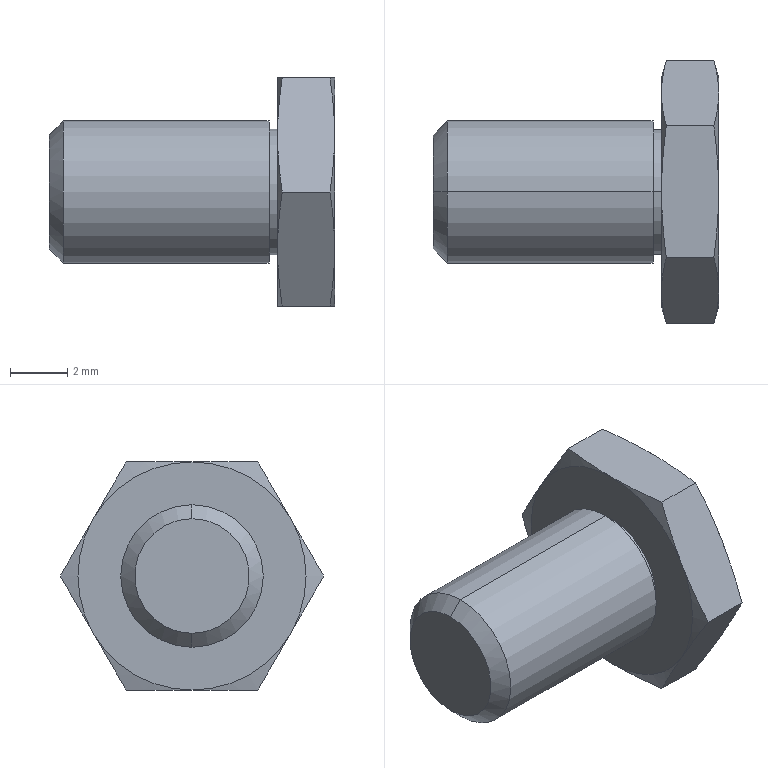Part | NX | features BREP 1 | 1 solid | 28 faces | box 10 x 9.238 x 8 mm | volume 264.32 mm3 | cone 14 | plane 10 | cylinder 4 | commonest cylinder face diameters 4.4 x2 5 x2
STEP:
#1=CARTESIAN_POINT('',(-7.51,0.,-2.5));
#2=VERTEX_POINT('',#1);
#3=CARTESIAN_POINT('',(-7.51,0.,2.5));
#4=VERTEX_POINT('',#3);
#5=CARTESIAN_POINT('',(-7.51,0.,0.));
#6=DIRECTION('',(1.,0.,0.));
#7=DIRECTION('',(0.,0.,-1.));
#8=AXIS2_PLACEMENT_3D('',#5,#6,#7);
#9=CIRCLE('',#8,2.5);
#10=EDGE_CURVE('',#2,#4,#9,.T.);
#11=ORIENTED_EDGE('',*,*,#10,.T.);
#12=CARTESIAN_POINT('',(-0.3,0.,2.5));
#13=VERTEX_POINT('',#12);
#14=CARTESIAN_POINT('',(-3.905,0.,2.5));
#15=DIRECTION('',(1.,0.,0.));
#16=VECTOR('',#15,1000.);
#17=LINE('',#14,#16);
#18=EDGE_CURVE('',#4,#13,#17,.T.);
#19=ORIENTED_EDGE('',*,*,#18,.T.);
#20=CARTESIAN_POINT('',(-0.3,0.,-2.5));
#21=VERTEX_POINT('',#20);
#22=CARTESIAN_POINT('',(-0.3,0.,0.));
#23=DIRECTION('',(-1.,0.,0.));
#24=DIRECTION('',(0.,0.,-1.));
#25=AXIS2_PLACEMENT_3D('',#22,#23,#24);
#26=CIRCLE('',#25,2.5);
#27=EDGE_CURVE('',#13,#21,#26,.T.);
#28=ORIENTED_EDGE('',*,*,#27,.T.);
#29=CARTESIAN_POINT('',(-3.905,0.,-2.5));
#30=DIRECTION('',(1.,0.,0.));
#31=VECTOR('',#30,1000.);
#32=LINE('',#29,#31);
#33=EDGE_CURVE('',#2,#21,#32,.T.);
#34=ORIENTED_EDGE('',*,*,#33,.F.);
#35=EDGE_LOOP('',(#11,#19,#28,#34));
#36=FACE_BOUND('',#35,.T.);
#37=CARTESIAN_POINT('',(-3.905,0.,0.));
#38=DIRECTION('',(1.,0.,0.));
#39=DIRECTION('',(0.,0.,-1.));
#40=AXIS2_PLACEMENT_3D('',#37,#38,#39);
#41=CYLINDRICAL_SURFACE('',#40,2.5);
#42=ADVANCED_FACE('',(#36),#41,.T.);
#43=CARTESIAN_POINT('',(-8.,0.,-2.009));
#44=VERTEX_POINT('',#43);
#45=CARTESIAN_POINT('',(-8.,0.,2.009));
#46=VERTEX_POINT('',#45);
#47=CARTESIAN_POINT('',(-8.,0.,0.));
#48=DIRECTION('',(1.,0.,0.));
#49=DIRECTION('',(0.,0.,-1.));
#50=AXIS2_PLACEMENT_3D('',#47,#48,#49);
#51=CIRCLE('',#50,2.009);
#52=EDGE_CURVE('',#44,#46,#51,.T.);
#53=ORIENTED_EDGE('',*,*,#52,.T.);
#54=CARTESIAN_POINT('',(-7.51,0.,2.5));
#55=DIRECTION('',(0.7071,0.,0.7071));
#56=VECTOR('',#55,1000.);
#57=LINE('',#54,#56);
#58=EDGE_CURVE('',#46,#4,#57,.T.);
#59=ORIENTED_EDGE('',*,*,#58,.T.);
#60=ORIENTED_EDGE('',*,*,#10,.F.);
#61=CARTESIAN_POINT('',(-7.51,0.,-2.5));
#62=DIRECTION('',(0.7071,0.,-0.7071));
#63=VECTOR('',#62,1000.);
#64=LINE('',#61,#63);
#65=EDGE_CURVE('',#44,#2,#64,.T.);
#66=ORIENTED_EDGE('',*,*,#65,.F.);
#67=EDGE_LOOP('',(#53,#59,#60,#66));
#68=FACE_BOUND('',#67,.T.);
#69=CARTESIAN_POINT('',(-7.51,0.,0.));
#70=DIRECTION('',(1.,0.,0.));
#71=DIRECTION('',(0.,0.,-1.));
#72=AXIS2_PLACEMENT_3D('',#69,#70,#71);
#73=CONICAL_SURFACE('',#72,2.5,0.7854);
#74=ADVANCED_FACE('',(#68),#73,.T.);
#75=CARTESIAN_POINT('',(-0.3,0.,2.2));
#76=VERTEX_POINT('',#75);
#77=CARTESIAN_POINT('',(-0.3,0.,-2.2));
#78=VERTEX_POINT('',#77);
#79=CARTESIAN_POINT('',(-0.3,0.,0.));
#80=DIRECTION('',(-1.,0.,0.));
#81=DIRECTION('',(0.,0.,-1.));
#82=AXIS2_PLACEMENT_3D('',#79,#80,#81);
#83=CIRCLE('',#82,2.2);
#84=EDGE_CURVE('',#76,#78,#83,.T.);
#85=ORIENTED_EDGE('',*,*,#84,.F.);
#86=CARTESIAN_POINT('',(0.,0.,2.2));
#87=VERTEX_POINT('',#86);
#88=CARTESIAN_POINT('',(-0.15,0.,2.2));
#89=DIRECTION('',(1.,0.,0.));
#90=VECTOR('',#89,1000.);
#91=LINE('',#88,#90);
#92=EDGE_CURVE('',#76,#87,#91,.T.);
#93=ORIENTED_EDGE('',*,*,#92,.T.);
#94=CARTESIAN_POINT('',(0.,0.,-2.2));
#95=VERTEX_POINT('',#94);
#96=CARTESIAN_POINT('',(0.,0.,0.));
#97=DIRECTION('',(-1.,0.,0.));
#98=DIRECTION('',(0.,0.,-1.));
#99=AXIS2_PLACEMENT_3D('',#96,#97,#98);
#100=CIRCLE('',#99,2.2);
#101=EDGE_CURVE('',#87,#95,#100,.T.);
#102=ORIENTED_EDGE('',*,*,#101,.T.);
#103=CARTESIAN_POINT('',(-0.15,0.,-2.2));
#104=DIRECTION('',(1.,0.,0.));
#105=VECTOR('',#104,1000.);
#106=LINE('',#103,#105);
#107=EDGE_CURVE('',#78,#95,#106,.T.);
#108=ORIENTED_EDGE('',*,*,#107,.F.);
#109=EDGE_LOOP('',(#85,#93,#102,#108));
#110=FACE_BOUND('',#109,.T.);
#111=CARTESIAN_POINT('',(-0.15,0.,0.));
#112=DIRECTION('',(1.,0.,0.));
#113=DIRECTION('',(0.,0.,-1.));
#114=AXIS2_PLACEMENT_3D('',#111,#112,#113);
#115=CYLINDRICAL_SURFACE('',#114,2.2);
#116=ADVANCED_FACE('',(#110),#115,.T.);
#117=ORIENTED_EDGE('',*,*,#18,.F.);
#118=CARTESIAN_POINT('',(-7.51,0.,0.));
#119=DIRECTION('',(1.,0.,0.));
#120=DIRECTION('',(0.,0.,-1.));
#121=AXIS2_PLACEMENT_3D('',#118,#119,#120);
#122=CIRCLE('',#121,2.5);
#123=EDGE_CURVE('',#4,#2,#122,.T.);
#124=ORIENTED_EDGE('',*,*,#123,.T.);
#125=ORIENTED_EDGE('',*,*,#33,.T.);
#126=CARTESIAN_POINT('',(-0.3,0.,0.));
#127=DIRECTION('',(-1.,0.,0.));
#128=DIRECTION('',(0.,0.,-1.));
#129=AXIS2_PLACEMENT_3D('',#126,#127,#128);
#130=CIRCLE('',#129,2.5);
#131=EDGE_CURVE('',#21,#13,#130,.T.);
#132=ORIENTED_EDGE('',*,*,#131,.T.);
#133=EDGE_LOOP('',(#117,#124,#125,#132));
#134=FACE_BOUND('',#133,.T.);
#135=CARTESIAN_POINT('',(-3.905,0.,0.));
#136=DIRECTION('',(1.,0.,0.));
#137=DIRECTION('',(0.,0.,-1.));
#138=AXIS2_PLACEMENT_3D('',#135,#136,#137);
#139=CYLINDRICAL_SURFACE('',#138,2.5);
#140=ADVANCED_FACE('',(#134),#139,.T.);
#141=ORIENTED_EDGE('',*,*,#58,.F.);
#142=CARTESIAN_POINT('',(-8.,0.,0.));
#143=DIRECTION('',(1.,0.,0.));
#144=DIRECTION('',(0.,0.,-1.));
#145=AXIS2_PLACEMENT_3D('',#142,#143,#144);
#146=CIRCLE('',#145,2.009);
#147=EDGE_CURVE('',#46,#44,#146,.T.);
#148=ORIENTED_EDGE('',*,*,#147,.T.);
#149=ORIENTED_EDGE('',*,*,#65,.T.);
#150=ORIENTED_EDGE('',*,*,#123,.F.);
#151=EDGE_LOOP('',(#141,#148,#149,#150));
#152=FACE_BOUND('',#151,.T.);
#153=CARTESIAN_POINT('',(-7.51,0.,0.));
#154=DIRECTION('',(1.,0.,0.));
#155=DIRECTION('',(0.,0.,-1.));
#156=AXIS2_PLACEMENT_3D('',#153,#154,#155);
#157=CONICAL_SURFACE('',#156,2.5,0.7854);
#158=ADVANCED_FACE('',(#152),#157,.T.);
#159=ORIENTED_EDGE('',*,*,#131,.F.);
#160=ORIENTED_EDGE('',*,*,#27,.F.);
#161=EDGE_LOOP('',(#159,#160));
#162=FACE_BOUND('',#161,.T.);
#163=CARTESIAN_POINT('',(-0.3,0.,0.));
#164=DIRECTION('',(-1.,0.,0.));
#165=DIRECTION('',(0.,0.,-1.));
#166=AXIS2_PLACEMENT_3D('',#163,#164,#165);
#167=CIRCLE('',#166,2.2);
#168=EDGE_CURVE('',#78,#76,#167,.T.);
#169=ORIENTED_EDGE('',*,*,#168,.T.);
#170=ORIENTED_EDGE('',*,*,#84,.T.);
#171=EDGE_LOOP('',(#169,#170));
#172=FACE_BOUND('',#171,.T.);
#173=CARTESIAN_POINT('',(-0.3,2.35,0.));
#174=DIRECTION('',(1.,0.,0.));
#175=DIRECTION('',(0.,-1.,0.));
#176=AXIS2_PLACEMENT_3D('',#173,#174,#175);
#177=PLANE('',#176);
#178=ADVANCED_FACE('',(#162,#172),#177,.T.);
#179=ORIENTED_EDGE('',*,*,#52,.F.);
#180=ORIENTED_EDGE('',*,*,#147,.F.);
#181=EDGE_LOOP('',(#179,#180));
#182=FACE_BOUND('',#181,.T.);
#183=CARTESIAN_POINT('',(-8.,1.005,0.));
#184=DIRECTION('',(-1.,0.,0.));
#185=DIRECTION('',(0.,0.,1.));
#186=AXIS2_PLACEMENT_3D('',#183,#184,#185);
#187=PLANE('',#186);
#188=ADVANCED_FACE('',(#182),#187,.T.);
#189=ORIENTED_EDGE('',*,*,#92,.F.);
#190=ORIENTED_EDGE('',*,*,#168,.F.);
#191=ORIENTED_EDGE('',*,*,#107,.T.);
#192=CARTESIAN_POINT('',(0.,0.,0.));
#193=DIRECTION('',(-1.,0.,0.));
#194=DIRECTION('',(0.,0.,-1.));
#195=AXIS2_PLACEMENT_3D('',#192,#193,#194);
#196=CIRCLE('',#195,2.2);
#197=EDGE_CURVE('',#95,#87,#196,.T.);
#198=ORIENTED_EDGE('',*,*,#197,.T.);
#199=EDGE_LOOP('',(#189,#190,#191,#198));
#200=FACE_BOUND('',#199,.T.);
#201=CARTESIAN_POINT('',(-0.15,0.,0.));
#202=DIRECTION('',(1.,0.,0.));
#203=DIRECTION('',(0.,0.,-1.));
#204=AXIS2_PLACEMENT_3D('',#201,#202,#203);
#205=CYLINDRICAL_SURFACE('',#204,2.2);
#206=ADVANCED_FACE('',(#200),#205,.T.);
#207=CARTESIAN_POINT('',(0.,-3.464,2.));
#208=VERTEX_POINT('',#207);
#209=CARTESIAN_POINT('',(0.,0.,4.));
#210=VERTEX_POINT('',#209);
#211=CARTESIAN_POINT('',(0.,0.,0.));
#212=DIRECTION('',(-1.,0.,0.));
#213=DIRECTION('',(0.,0.,-1.));
#214=AXIS2_PLACEMENT_3D('',#211,#212,#213);
#215=CIRCLE('',#214,4.);
#216=EDGE_CURVE('',#208,#210,#215,.T.);
#217=ORIENTED_EDGE('',*,*,#216,.T.);
#218=CARTESIAN_POINT('',(0.,3.464,2.));
#219=VERTEX_POINT('',#218);
#220=CARTESIAN_POINT('',(0.,0.,0.));
#221=DIRECTION('',(-1.,0.,0.));
#222=DIRECTION('',(0.,0.,-1.));
#223=AXIS2_PLACEMENT_3D('',#220,#221,#222);
#224=CIRCLE('',#223,4.);
#225=EDGE_CURVE('',#210,#219,#224,.T.);
#226=ORIENTED_EDGE('',*,*,#225,.T.);
#227=CARTESIAN_POINT('',(0.,3.464,-2.));
#228=VERTEX_POINT('',#227);
#229=CARTESIAN_POINT('',(0.,0.,0.));
#230=DIRECTION('',(-1.,0.,0.));
#231=DIRECTION('',(0.,0.,-1.));
#232=AXIS2_PLACEMENT_3D('',#229,#230,#231);
#233=CIRCLE('',#232,4.);
#234=EDGE_CURVE('',#219,#228,#233,.T.);
#235=ORIENTED_EDGE('',*,*,#234,.T.);
#236=CARTESIAN_POINT('',(0.,0.,-4.));
#237=VERTEX_POINT('',#236);
#238=CARTESIAN_POINT('',(0.,0.,0.));
#239=DIRECTION('',(-1.,0.,0.));
#240=DIRECTION('',(0.,0.,-1.));
#241=AXIS2_PLACEMENT_3D('',#238,#239,#240);
#242=CIRCLE('',#241,4.);
#243=EDGE_CURVE('',#228,#237,#242,.T.);
#244=ORIENTED_EDGE('',*,*,#243,.T.);
#245=CARTESIAN_POINT('',(0.,-3.464,-2.));
#246=VERTEX_POINT('',#245);
#247=CARTESIAN_POINT('',(0.,0.,0.));
#248=DIRECTION('',(-1.,0.,0.));
#249=DIRECTION('',(0.,0.,-1.));
#250=AXIS2_PLACEMENT_3D('',#247,#248,#249);
#251=CIRCLE('',#250,4.);
#252=EDGE_CURVE('',#237,#246,#251,.T.);
#253=ORIENTED_EDGE('',*,*,#252,.T.);
#254=CARTESIAN_POINT('',(0.,0.,0.));
#255=DIRECTION('',(-1.,0.,0.));
#256=DIRECTION('',(0.,0.,-1.));
#257=AXIS2_PLACEMENT_3D('',#254,#255,#256);
#258=CIRCLE('',#257,4.);
#259=EDGE_CURVE('',#246,#208,#258,.T.);
#260=ORIENTED_EDGE('',*,*,#259,.T.);
#261=EDGE_LOOP('',(#217,#226,#235,#244,#253,#260));
#262=FACE_BOUND('',#261,.T.);
#263=ORIENTED_EDGE('',*,*,#197,.F.);
#264=ORIENTED_EDGE('',*,*,#101,.F.);
#265=EDGE_LOOP('',(#263,#264));
#266=FACE_BOUND('',#265,.T.);
#267=CARTESIAN_POINT('',(0.,2.,0.));
#268=DIRECTION('',(-1.,0.,0.));
#269=DIRECTION('',(0.,0.,1.));
#270=AXIS2_PLACEMENT_3D('',#267,#268,#269);
#271=PLANE('',#270);
#272=ADVANCED_FACE('',(#262,#266),#271,.T.);
#273=CARTESIAN_POINT('',(0.1658,2.309,4.));
#274=VERTEX_POINT('',#273);
#275=CARTESIAN_POINT('',(0.,3.464,2.));
#276=CARTESIAN_POINT('',(0.,3.086,2.654));
#277=CARTESIAN_POINT('',(0.05761,2.713,3.301));
#278=CARTESIAN_POINT('',(0.1658,2.309,4.));
#279=B_SPLINE_CURVE_WITH_KNOTS('',3,(#275,#276,#277,#278),.UNSPECIFIED.,.F.,.F.,(4,4),(0.,1.),.UNSPECIFIED.);
#280=EDGE_CURVE('',#274,#219,#279,.F.);
#281=ORIENTED_EDGE('',*,*,#280,.T.);
#282=ORIENTED_EDGE('',*,*,#225,.F.);
#283=CARTESIAN_POINT('',(0.1658,2.309,4.));
#284=CARTESIAN_POINT('',(0.0577,1.502,4.));
#285=CARTESIAN_POINT('',(0.,0.7558,4.));
#286=CARTESIAN_POINT('',(0.,0.,4.));
#287=B_SPLINE_CURVE_WITH_KNOTS('',3,(#283,#284,#285,#286),.UNSPECIFIED.,.F.,.F.,(4,4),(0.,1.),.UNSPECIFIED.);
#288=EDGE_CURVE('',#210,#274,#287,.F.);
#289=ORIENTED_EDGE('',*,*,#288,.T.);
#290=EDGE_LOOP('',(#281,#282,#289));
#291=FACE_BOUND('',#290,.T.);
#292=CARTESIAN_POINT('',(0.1668,0.,0.));
#293=DIRECTION('',(1.,0.,0.));
#294=DIRECTION('',(0.,0.,-1.));
#295=AXIS2_PLACEMENT_3D('',#292,#293,#294);
#296=CONICAL_SURFACE('',#295,4.623,1.309);
#297=ADVANCED_FACE('',(#291),#296,.T.);
#298=CARTESIAN_POINT('',(0.1658,-2.309,4.));
#299=VERTEX_POINT('',#298);
#300=CARTESIAN_POINT('',(0.,0.,4.));
#301=CARTESIAN_POINT('',(0.,-0.7553,4.));
#302=CARTESIAN_POINT('',(0.05761,-1.502,4.));
#303=CARTESIAN_POINT('',(0.1658,-2.309,4.));
#304=B_SPLINE_CURVE_WITH_KNOTS('',3,(#300,#301,#302,#303),.UNSPECIFIED.,.F.,.F.,(4,4),(0.,1.),.UNSPECIFIED.);
#305=EDGE_CURVE('',#299,#210,#304,.F.);
#306=ORIENTED_EDGE('',*,*,#305,.T.);
#307=ORIENTED_EDGE('',*,*,#216,.F.);
#308=CARTESIAN_POINT('',(0.1658,-2.309,4.));
#309=CARTESIAN_POINT('',(0.0577,-2.713,3.301));
#310=CARTESIAN_POINT('',(0.,-3.086,2.655));
#311=CARTESIAN_POINT('',(0.,-3.464,2.));
#312=B_SPLINE_CURVE_WITH_KNOTS('',3,(#308,#309,#310,#311),.UNSPECIFIED.,.F.,.F.,(4,4),(0.,1.),.UNSPECIFIED.);
#313=EDGE_CURVE('',#208,#299,#312,.F.);
#314=ORIENTED_EDGE('',*,*,#313,.T.);
#315=EDGE_LOOP('',(#306,#307,#314));
#316=FACE_BOUND('',#315,.T.);
#317=CARTESIAN_POINT('',(0.1668,0.,0.));
#318=DIRECTION('',(1.,0.,0.));
#319=DIRECTION('',(0.,0.,-1.));
#320=AXIS2_PLACEMENT_3D('',#317,#318,#319);
#321=CONICAL_SURFACE('',#320,4.623,1.309);
#322=ADVANCED_FACE('',(#316),#321,.T.);
#323=CARTESIAN_POINT('',(0.1658,-4.619,0.));
#324=VERTEX_POINT('',#323);
#325=CARTESIAN_POINT('',(0.,-3.464,2.));
#326=CARTESIAN_POINT('',(0.,-3.842,1.346));
#327=CARTESIAN_POINT('',(0.05761,-4.215,0.6994));
#328=CARTESIAN_POINT('',(0.1658,-4.619,0.));
#329=B_SPLINE_CURVE_WITH_KNOTS('',3,(#325,#326,#327,#328),.UNSPECIFIED.,.F.,.F.,(4,4),(0.,1.),.UNSPECIFIED.);
#330=EDGE_CURVE('',#324,#208,#329,.F.);
#331=ORIENTED_EDGE('',*,*,#330,.T.);
#332=ORIENTED_EDGE('',*,*,#259,.F.);
#333=CARTESIAN_POINT('',(0.1658,-4.619,0.));
#334=CARTESIAN_POINT('',(0.0577,-4.215,-0.6988));
#335=CARTESIAN_POINT('',(0.,-3.842,-1.345));
#336=CARTESIAN_POINT('',(0.,-3.464,-2.));
#337=B_SPLINE_CURVE_WITH_KNOTS('',3,(#333,#334,#335,#336),.UNSPECIFIED.,.F.,.F.,(4,4),(0.,1.),.UNSPECIFIED.);
#338=EDGE_CURVE('',#246,#324,#337,.F.);
#339=ORIENTED_EDGE('',*,*,#338,.T.);
#340=EDGE_LOOP('',(#331,#332,#339));
#341=FACE_BOUND('',#340,.T.);
#342=CARTESIAN_POINT('',(0.1668,0.,0.));
#343=DIRECTION('',(1.,0.,0.));
#344=DIRECTION('',(0.,0.,-1.));
#345=AXIS2_PLACEMENT_3D('',#342,#343,#344);
#346=CONICAL_SURFACE('',#345,4.623,1.309);
#347=ADVANCED_FACE('',(#341),#346,.T.);
#348=ORIENTED_EDGE('',*,*,#252,.F.);
#349=CARTESIAN_POINT('',(0.1658,-2.309,-4.));
#350=VERTEX_POINT('',#349);
#351=CARTESIAN_POINT('',(0.1658,-2.309,-4.));
#352=CARTESIAN_POINT('',(0.0577,-1.502,-4.));
#353=CARTESIAN_POINT('',(0.,-0.7558,-4.));
#354=CARTESIAN_POINT('',(0.,0.,-4.));
#355=B_SPLINE_CURVE_WITH_KNOTS('',3,(#351,#352,#353,#354),.UNSPECIFIED.,.F.,.F.,(4,4),(0.,1.),.UNSPECIFIED.);
#356=EDGE_CURVE('',#237,#350,#355,.F.);
#357=ORIENTED_EDGE('',*,*,#356,.T.);
#358=CARTESIAN_POINT('',(0.,-3.464,-2.));
#359=CARTESIAN_POINT('',(0.,-3.086,-2.654));
#360=CARTESIAN_POINT('',(0.05761,-2.713,-3.301));
#361=CARTESIAN_POINT('',(0.1658,-2.309,-4.));
#362=B_SPLINE_CURVE_WITH_KNOTS('',3,(#358,#359,#360,#361),.UNSPECIFIED.,.F.,.F.,(4,4),(0.,1.),.UNSPECIFIED.);
#363=EDGE_CURVE('',#350,#246,#362,.F.);
#364=ORIENTED_EDGE('',*,*,#363,.T.);
#365=EDGE_LOOP('',(#348,#357,#364));
#366=FACE_BOUND('',#365,.T.);
#367=CARTESIAN_POINT('',(0.1668,0.,0.));
#368=DIRECTION('',(1.,0.,0.));
#369=DIRECTION('',(0.,0.,-1.));
#370=AXIS2_PLACEMENT_3D('',#367,#368,#369);
#371=CONICAL_SURFACE('',#370,4.623,1.309);
#372=ADVANCED_FACE('',(#366),#371,.T.);
#373=ORIENTED_EDGE('',*,*,#243,.F.);
#374=CARTESIAN_POINT('',(0.1658,2.309,-4.));
#375=VERTEX_POINT('',#374);
#376=CARTESIAN_POINT('',(0.1658,2.309,-4.));
#377=CARTESIAN_POINT('',(0.0577,2.713,-3.301));
#378=CARTESIAN_POINT('',(0.,3.086,-2.655));
#379=CARTESIAN_POINT('',(0.,3.464,-2.));
#380=B_SPLINE_CURVE_WITH_KNOTS('',3,(#376,#377,#378,#379),.UNSPECIFIED.,.F.,.F.,(4,4),(0.,1.),.UNSPECIFIED.);
#381=EDGE_CURVE('',#228,#375,#380,.F.);
#382=ORIENTED_EDGE('',*,*,#381,.T.);
#383=CARTESIAN_POINT('',(0.,0.,-4.));
#384=CARTESIAN_POINT('',(0.,0.7553,-4.));
#385=CARTESIAN_POINT('',(0.05761,1.502,-4.));
#386=CARTESIAN_POINT('',(0.1658,2.309,-4.));
#387=B_SPLINE_CURVE_WITH_KNOTS('',3,(#383,#384,#385,#386),.UNSPECIFIED.,.F.,.F.,(4,4),(0.,1.),.UNSPECIFIED.);
#388=EDGE_CURVE('',#375,#237,#387,.F.);
#389=ORIENTED_EDGE('',*,*,#388,.T.);
#390=EDGE_LOOP('',(#373,#382,#389));
#391=FACE_BOUND('',#390,.T.);
#392=CARTESIAN_POINT('',(0.1668,0.,0.));
#393=DIRECTION('',(1.,0.,0.));
#394=DIRECTION('',(0.,0.,-1.));
#395=AXIS2_PLACEMENT_3D('',#392,#393,#394);
#396=CONICAL_SURFACE('',#395,4.623,1.309);
#397=ADVANCED_FACE('',(#391),#396,.T.);
#398=CARTESIAN_POINT('',(0.1658,4.619,0.));
#399=VERTEX_POINT('',#398);
#400=CARTESIAN_POINT('',(0.,3.464,-2.));
#401=CARTESIAN_POINT('',(0.,3.842,-1.346));
#402=CARTESIAN_POINT('',(0.05761,4.215,-0.6994));
#403=CARTESIAN_POINT('',(0.1658,4.619,0.));
#404=B_SPLINE_CURVE_WITH_KNOTS('',3,(#400,#401,#402,#403),.UNSPECIFIED.,.F.,.F.,(4,4),(0.,1.),.UNSPECIFIED.);
#405=EDGE_CURVE('',#399,#228,#404,.F.);
#406=ORIENTED_EDGE('',*,*,#405,.T.);
#407=ORIENTED_EDGE('',*,*,#234,.F.);
#408=CARTESIAN_POINT('',(0.1658,4.619,0.));
#409=CARTESIAN_POINT('',(0.0577,4.215,0.6988));
#410=CARTESIAN_POINT('',(0.,3.842,1.345));
#411=CARTESIAN_POINT('',(0.,3.464,2.));
#412=B_SPLINE_CURVE_WITH_KNOTS('',3,(#408,#409,#410,#411),.UNSPECIFIED.,.F.,.F.,(4,4),(0.,1.),.UNSPECIFIED.);
#413=EDGE_CURVE('',#219,#399,#412,.F.);
#414=ORIENTED_EDGE('',*,*,#413,.T.);
#415=EDGE_LOOP('',(#406,#407,#414));
#416=FACE_BOUND('',#415,.T.);
#417=CARTESIAN_POINT('',(0.1668,0.,0.));
#418=DIRECTION('',(1.,0.,0.));
#419=DIRECTION('',(0.,0.,-1.));
#420=AXIS2_PLACEMENT_3D('',#417,#418,#419);
#421=CONICAL_SURFACE('',#420,4.623,1.309);
#422=ADVANCED_FACE('',(#416),#421,.T.);
#423=CARTESIAN_POINT('',(1.834,4.619,0.));
#424=VERTEX_POINT('',#423);
#425=CARTESIAN_POINT('',(0.,4.619,0.));
#426=DIRECTION('',(1.,0.,0.));
#427=VECTOR('',#426,1000.);
#428=LINE('',#425,#427);
#429=EDGE_CURVE('',#399,#424,#428,.T.);
#430=ORIENTED_EDGE('',*,*,#429,.F.);
#431=ORIENTED_EDGE('',*,*,#413,.F.);
#432=ORIENTED_EDGE('',*,*,#280,.F.);
#433=CARTESIAN_POINT('',(1.834,2.309,4.));
#434=VERTEX_POINT('',#433);
#435=CARTESIAN_POINT('',(0.,2.309,4.));
#436=DIRECTION('',(-1.,0.,0.));
#437=VECTOR('',#436,1000.);
#438=LINE('',#435,#437);
#439=EDGE_CURVE('',#434,#274,#438,.T.);
#440=ORIENTED_EDGE('',*,*,#439,.F.);
#441=CARTESIAN_POINT('',(2.,3.464,2.));
#442=VERTEX_POINT('',#441);
#443=CARTESIAN_POINT('',(1.834,2.309,4.));
#444=CARTESIAN_POINT('',(1.942,2.713,3.301));
#445=CARTESIAN_POINT('',(2.,3.086,2.655));
#446=CARTESIAN_POINT('',(2.,3.464,2.));
#447=B_SPLINE_CURVE_WITH_KNOTS('',3,(#443,#444,#445,#446),.UNSPECIFIED.,.F.,.F.,(4,4),(0.,1.),.UNSPECIFIED.);
#448=EDGE_CURVE('',#442,#434,#447,.F.);
#449=ORIENTED_EDGE('',*,*,#448,.F.);
#450=CARTESIAN_POINT('',(2.,3.464,2.));
#451=CARTESIAN_POINT('',(2.,3.842,1.346));
#452=CARTESIAN_POINT('',(1.942,4.215,0.6994));
#453=CARTESIAN_POINT('',(1.834,4.619,0.));
#454=B_SPLINE_CURVE_WITH_KNOTS('',3,(#450,#451,#452,#453),.UNSPECIFIED.,.F.,.F.,(4,4),(0.,1.),.UNSPECIFIED.);
#455=EDGE_CURVE('',#424,#442,#454,.F.);
#456=ORIENTED_EDGE('',*,*,#455,.F.);
#457=EDGE_LOOP('',(#430,#431,#432,#440,#449,#456));
#458=FACE_BOUND('',#457,.T.);
#459=CARTESIAN_POINT('',(0.,4.619,0.));
#460=DIRECTION('',(0.,-0.866,-0.5));
#461=DIRECTION('',(0.,0.5,-0.866));
#462=AXIS2_PLACEMENT_3D('',#459,#460,#461);
#463=PLANE('',#462);
#464=ADVANCED_FACE('',(#458),#463,.F.);
#465=CARTESIAN_POINT('',(2.,0.,4.));
#466=VERTEX_POINT('',#465);
#467=CARTESIAN_POINT('',(2.,0.,4.));
#468=CARTESIAN_POINT('',(2.,0.7553,4.));
#469=CARTESIAN_POINT('',(1.942,1.502,4.));
#470=CARTESIAN_POINT('',(1.834,2.309,4.));
#471=B_SPLINE_CURVE_WITH_KNOTS('',3,(#467,#468,#469,#470),.UNSPECIFIED.,.F.,.F.,(4,4),(0.,1.),.UNSPECIFIED.);
#472=EDGE_CURVE('',#434,#466,#471,.F.);
#473=ORIENTED_EDGE('',*,*,#472,.F.);
#474=ORIENTED_EDGE('',*,*,#439,.T.);
#475=ORIENTED_EDGE('',*,*,#288,.F.);
#476=ORIENTED_EDGE('',*,*,#305,.F.);
#477=CARTESIAN_POINT('',(1.834,-2.309,4.));
#478=VERTEX_POINT('',#477);
#479=CARTESIAN_POINT('',(0.,-2.309,4.));
#480=DIRECTION('',(-1.,0.,0.));
#481=VECTOR('',#480,1000.);
#482=LINE('',#479,#481);
#483=EDGE_CURVE('',#478,#299,#482,.T.);
#484=ORIENTED_EDGE('',*,*,#483,.F.);
#485=CARTESIAN_POINT('',(1.834,-2.309,4.));
#486=CARTESIAN_POINT('',(1.942,-1.502,4.));
#487=CARTESIAN_POINT('',(2.,-0.7558,4.));
#488=CARTESIAN_POINT('',(2.,0.,4.));
#489=B_SPLINE_CURVE_WITH_KNOTS('',3,(#485,#486,#487,#488),.UNSPECIFIED.,.F.,.F.,(4,4),(0.,1.),.UNSPECIFIED.);
#490=EDGE_CURVE('',#466,#478,#489,.F.);
#491=ORIENTED_EDGE('',*,*,#490,.F.);
#492=EDGE_LOOP('',(#473,#474,#475,#476,#484,#491));
#493=FACE_BOUND('',#492,.T.);
#494=CARTESIAN_POINT('',(0.,2.309,4.));
#495=DIRECTION('',(0.,0.,-1.));
#496=DIRECTION('',(0.,-1.,0.));
#497=AXIS2_PLACEMENT_3D('',#494,#495,#496);
#498=PLANE('',#497);
#499=ADVANCED_FACE('',(#493),#498,.F.);
#500=CARTESIAN_POINT('',(2.,-3.464,2.));
#501=VERTEX_POINT('',#500);
#502=CARTESIAN_POINT('',(2.,-3.464,2.));
#503=CARTESIAN_POINT('',(2.,-3.086,2.654));
#504=CARTESIAN_POINT('',(1.942,-2.713,3.301));
#505=CARTESIAN_POINT('',(1.834,-2.309,4.));
#506=B_SPLINE_CURVE_WITH_KNOTS('',3,(#502,#503,#504,#505),.UNSPECIFIED.,.F.,.F.,(4,4),(0.,1.),.UNSPECIFIED.);
#507=EDGE_CURVE('',#478,#501,#506,.F.);
#508=ORIENTED_EDGE('',*,*,#507,.F.);
#509=ORIENTED_EDGE('',*,*,#483,.T.);
#510=ORIENTED_EDGE('',*,*,#313,.F.);
#511=ORIENTED_EDGE('',*,*,#330,.F.);
#512=CARTESIAN_POINT('',(1.834,-4.619,0.));
#513=VERTEX_POINT('',#512);
#514=CARTESIAN_POINT('',(0.,-4.619,0.));
#515=DIRECTION('',(-1.,0.,0.));
#516=VECTOR('',#515,1000.);
#517=LINE('',#514,#516);
#518=EDGE_CURVE('',#513,#324,#517,.T.);
#519=ORIENTED_EDGE('',*,*,#518,.F.);
#520=CARTESIAN_POINT('',(1.834,-4.619,0.));
#521=CARTESIAN_POINT('',(1.942,-4.215,0.6988));
#522=CARTESIAN_POINT('',(2.,-3.842,1.345));
#523=CARTESIAN_POINT('',(2.,-3.464,2.));
#524=B_SPLINE_CURVE_WITH_KNOTS('',3,(#520,#521,#522,#523),.UNSPECIFIED.,.F.,.F.,(4,4),(0.,1.),.UNSPECIFIED.);
#525=EDGE_CURVE('',#501,#513,#524,.F.);
#526=ORIENTED_EDGE('',*,*,#525,.F.);
#527=EDGE_LOOP('',(#508,#509,#510,#511,#519,#526));
#528=FACE_BOUND('',#527,.T.);
#529=CARTESIAN_POINT('',(0.,-2.309,4.));
#530=DIRECTION('',(0.,0.866,-0.5));
#531=DIRECTION('',(-1.,0.,0.));
#532=AXIS2_PLACEMENT_3D('',#529,#530,#531);
#533=PLANE('',#532);
#534=ADVANCED_FACE('',(#528),#533,.F.);
#535=CARTESIAN_POINT('',(2.,-3.464,-2.));
#536=VERTEX_POINT('',#535);
#537=CARTESIAN_POINT('',(2.,-3.464,-2.));
#538=CARTESIAN_POINT('',(2.,-3.842,-1.346));
#539=CARTESIAN_POINT('',(1.942,-4.215,-0.6994));
#540=CARTESIAN_POINT('',(1.834,-4.619,0.));
#541=B_SPLINE_CURVE_WITH_KNOTS('',3,(#537,#538,#539,#540),.UNSPECIFIED.,.F.,.F.,(4,4),(0.,1.),.UNSPECIFIED.);
#542=EDGE_CURVE('',#513,#536,#541,.F.);
#543=ORIENTED_EDGE('',*,*,#542,.F.);
#544=ORIENTED_EDGE('',*,*,#518,.T.);
#545=ORIENTED_EDGE('',*,*,#338,.F.);
#546=ORIENTED_EDGE('',*,*,#363,.F.);
#547=CARTESIAN_POINT('',(1.834,-2.309,-4.));
#548=VERTEX_POINT('',#547);
#549=CARTESIAN_POINT('',(0.,-2.309,-4.));
#550=DIRECTION('',(-1.,0.,0.));
#551=VECTOR('',#550,1000.);
#552=LINE('',#549,#551);
#553=EDGE_CURVE('',#548,#350,#552,.T.);
#554=ORIENTED_EDGE('',*,*,#553,.F.);
#555=CARTESIAN_POINT('',(1.834,-2.309,-4.));
#556=CARTESIAN_POINT('',(1.942,-2.713,-3.301));
#557=CARTESIAN_POINT('',(2.,-3.086,-2.655));
#558=CARTESIAN_POINT('',(2.,-3.464,-2.));
#559=B_SPLINE_CURVE_WITH_KNOTS('',3,(#555,#556,#557,#558),.UNSPECIFIED.,.F.,.F.,(4,4),(0.,1.),.UNSPECIFIED.);
#560=EDGE_CURVE('',#536,#548,#559,.F.);
#561=ORIENTED_EDGE('',*,*,#560,.F.);
#562=EDGE_LOOP('',(#543,#544,#545,#546,#554,#561));
#563=FACE_BOUND('',#562,.T.);
#564=CARTESIAN_POINT('',(0.,-4.619,0.));
#565=DIRECTION('',(0.,0.866,0.5));
#566=DIRECTION('',(1.,0.,0.));
#567=AXIS2_PLACEMENT_3D('',#564,#565,#566);
#568=PLANE('',#567);
#569=ADVANCED_FACE('',(#563),#568,.F.);
#570=ORIENTED_EDGE('',*,*,#553,.T.);
#571=ORIENTED_EDGE('',*,*,#356,.F.);
#572=ORIENTED_EDGE('',*,*,#388,.F.);
#573=CARTESIAN_POINT('',(1.834,2.309,-4.));
#574=VERTEX_POINT('',#573);
#575=CARTESIAN_POINT('',(0.,2.309,-4.));
#576=DIRECTION('',(-1.,0.,0.));
#577=VECTOR('',#576,1000.);
#578=LINE('',#575,#577);
#579=EDGE_CURVE('',#574,#375,#578,.T.);
#580=ORIENTED_EDGE('',*,*,#579,.F.);
#581=CARTESIAN_POINT('',(2.,0.,-4.));
#582=VERTEX_POINT('',#581);
#583=CARTESIAN_POINT('',(1.834,2.309,-4.));
#584=CARTESIAN_POINT('',(1.942,1.502,-4.));
#585=CARTESIAN_POINT('',(2.,0.7558,-4.));
#586=CARTESIAN_POINT('',(2.,0.,-4.));
#587=B_SPLINE_CURVE_WITH_KNOTS('',3,(#583,#584,#585,#586),.UNSPECIFIED.,.F.,.F.,(4,4),(0.,1.),.UNSPECIFIED.);
#588=EDGE_CURVE('',#582,#574,#587,.F.);
#589=ORIENTED_EDGE('',*,*,#588,.F.);
#590=CARTESIAN_POINT('',(2.,0.,-4.));
#591=CARTESIAN_POINT('',(2.,-0.7553,-4.));
#592=CARTESIAN_POINT('',(1.942,-1.502,-4.));
#593=CARTESIAN_POINT('',(1.834,-2.309,-4.));
#594=B_SPLINE_CURVE_WITH_KNOTS('',3,(#590,#591,#592,#593),.UNSPECIFIED.,.F.,.F.,(4,4),(0.,1.),.UNSPECIFIED.);
#595=EDGE_CURVE('',#548,#582,#594,.F.);
#596=ORIENTED_EDGE('',*,*,#595,.F.);
#597=EDGE_LOOP('',(#570,#571,#572,#580,#589,#596));
#598=FACE_BOUND('',#597,.T.);
#599=CARTESIAN_POINT('',(0.,-2.309,-4.));
#600=DIRECTION('',(0.,0.,1.));
#601=DIRECTION('',(1.,0.,0.));
#602=AXIS2_PLACEMENT_3D('',#599,#600,#601);
#603=PLANE('',#602);
#604=ADVANCED_FACE('',(#598),#603,.F.);
#605=ORIENTED_EDGE('',*,*,#579,.T.);
#606=ORIENTED_EDGE('',*,*,#381,.F.);
#607=ORIENTED_EDGE('',*,*,#405,.F.);
#608=ORIENTED_EDGE('',*,*,#429,.T.);
#609=CARTESIAN_POINT('',(2.,3.464,-2.));
#610=VERTEX_POINT('',#609);
#611=CARTESIAN_POINT('',(1.834,4.619,0.));
#612=CARTESIAN_POINT('',(1.942,4.215,-0.6988));
#613=CARTESIAN_POINT('',(2.,3.842,-1.345));
#614=CARTESIAN_POINT('',(2.,3.464,-2.));
#615=B_SPLINE_CURVE_WITH_KNOTS('',3,(#611,#612,#613,#614),.UNSPECIFIED.,.F.,.F.,(4,4),(0.,1.),.UNSPECIFIED.);
#616=EDGE_CURVE('',#610,#424,#615,.F.);
#617=ORIENTED_EDGE('',*,*,#616,.F.);
#618=CARTESIAN_POINT('',(2.,3.464,-2.));
#619=CARTESIAN_POINT('',(2.,3.086,-2.654));
#620=CARTESIAN_POINT('',(1.942,2.713,-3.301));
#621=CARTESIAN_POINT('',(1.834,2.309,-4.));
#622=B_SPLINE_CURVE_WITH_KNOTS('',3,(#618,#619,#620,#621),.UNSPECIFIED.,.F.,.F.,(4,4),(0.,1.),.UNSPECIFIED.);
#623=EDGE_CURVE('',#574,#610,#622,.F.);
#624=ORIENTED_EDGE('',*,*,#623,.F.);
#625=EDGE_LOOP('',(#605,#606,#607,#608,#617,#624));
#626=FACE_BOUND('',#625,.T.);
#627=CARTESIAN_POINT('',(0.,2.309,-4.));
#628=DIRECTION('',(0.,-0.866,0.5));
#629=DIRECTION('',(-1.,0.,0.));
#630=AXIS2_PLACEMENT_3D('',#627,#628,#629);
#631=PLANE('',#630);
#632=ADVANCED_FACE('',(#626),#631,.F.);
#633=ORIENTED_EDGE('',*,*,#455,.T.);
#634=CARTESIAN_POINT('',(2.,0.,0.));
#635=DIRECTION('',(-1.,0.,0.));
#636=DIRECTION('',(0.,0.,1.));
#637=AXIS2_PLACEMENT_3D('',#634,#635,#636);
#638=CIRCLE('',#637,4.);
#639=EDGE_CURVE('',#442,#610,#638,.T.);
#640=ORIENTED_EDGE('',*,*,#639,.T.);
#641=ORIENTED_EDGE('',*,*,#616,.T.);
#642=EDGE_LOOP('',(#633,#640,#641));
#643=FACE_BOUND('',#642,.T.);
#644=CARTESIAN_POINT('',(1.833,0.,0.));
#645=DIRECTION('',(-1.,0.,0.));
#646=DIRECTION('',(0.,0.,1.));
#647=AXIS2_PLACEMENT_3D('',#644,#645,#646);
#648=CONICAL_SURFACE('',#647,4.623,1.309);
#649=ADVANCED_FACE('',(#643),#648,.T.);
#650=ORIENTED_EDGE('',*,*,#472,.T.);
#651=CARTESIAN_POINT('',(2.,0.,0.));
#652=DIRECTION('',(-1.,0.,0.));
#653=DIRECTION('',(0.,0.,1.));
#654=AXIS2_PLACEMENT_3D('',#651,#652,#653);
#655=CIRCLE('',#654,4.);
#656=EDGE_CURVE('',#466,#442,#655,.T.);
#657=ORIENTED_EDGE('',*,*,#656,.T.);
#658=ORIENTED_EDGE('',*,*,#448,.T.);
#659=EDGE_LOOP('',(#650,#657,#658));
#660=FACE_BOUND('',#659,.T.);
#661=CARTESIAN_POINT('',(1.833,0.,0.));
#662=DIRECTION('',(-1.,0.,0.));
#663=DIRECTION('',(0.,0.,1.));
#664=AXIS2_PLACEMENT_3D('',#661,#662,#663);
#665=CONICAL_SURFACE('',#664,4.623,1.309);
#666=ADVANCED_FACE('',(#660),#665,.T.);
#667=CARTESIAN_POINT('',(2.,0.,0.));
#668=DIRECTION('',(-1.,0.,0.));
#669=DIRECTION('',(0.,0.,1.));
#670=AXIS2_PLACEMENT_3D('',#667,#668,#669);
#671=CIRCLE('',#670,4.);
#672=EDGE_CURVE('',#501,#466,#671,.T.);
#673=ORIENTED_EDGE('',*,*,#672,.T.);
#674=ORIENTED_EDGE('',*,*,#490,.T.);
#675=ORIENTED_EDGE('',*,*,#507,.T.);
#676=EDGE_LOOP('',(#673,#674,#675));
#677=FACE_BOUND('',#676,.T.);
#678=CARTESIAN_POINT('',(1.833,0.,0.));
#679=DIRECTION('',(-1.,0.,0.));
#680=DIRECTION('',(0.,0.,1.));
#681=AXIS2_PLACEMENT_3D('',#678,#679,#680);
#682=CONICAL_SURFACE('',#681,4.623,1.309);
#683=ADVANCED_FACE('',(#677),#682,.T.);
#684=CARTESIAN_POINT('',(2.,0.,0.));
#685=DIRECTION('',(-1.,0.,0.));
#686=DIRECTION('',(0.,0.,1.));
#687=AXIS2_PLACEMENT_3D('',#684,#685,#686);
#688=CIRCLE('',#687,4.);
#689=EDGE_CURVE('',#536,#501,#688,.T.);
#690=ORIENTED_EDGE('',*,*,#689,.T.);
#691=ORIENTED_EDGE('',*,*,#525,.T.);
#692=ORIENTED_EDGE('',*,*,#542,.T.);
#693=EDGE_LOOP('',(#690,#691,#692));
#694=FACE_BOUND('',#693,.T.);
#695=CARTESIAN_POINT('',(1.833,0.,0.));
#696=DIRECTION('',(-1.,0.,0.));
#697=DIRECTION('',(0.,0.,1.));
#698=AXIS2_PLACEMENT_3D('',#695,#696,#697);
#699=CONICAL_SURFACE('',#698,4.623,1.309);
#700=ADVANCED_FACE('',(#694),#699,.T.);
#701=CARTESIAN_POINT('',(2.,0.,0.));
#702=DIRECTION('',(-1.,0.,0.));
#703=DIRECTION('',(0.,0.,1.));
#704=AXIS2_PLACEMENT_3D('',#701,#702,#703);
#705=CIRCLE('',#704,4.);
#706=EDGE_CURVE('',#582,#536,#705,.T.);
#707=ORIENTED_EDGE('',*,*,#706,.T.);
#708=ORIENTED_EDGE('',*,*,#560,.T.);
#709=ORIENTED_EDGE('',*,*,#595,.T.);
#710=EDGE_LOOP('',(#707,#708,#709));
#711=FACE_BOUND('',#710,.T.);
#712=CARTESIAN_POINT('',(1.833,0.,0.));
#713=DIRECTION('',(-1.,0.,0.));
#714=DIRECTION('',(0.,0.,1.));
#715=AXIS2_PLACEMENT_3D('',#712,#713,#714);
#716=CONICAL_SURFACE('',#715,4.623,1.309);
#717=ADVANCED_FACE('',(#711),#716,.T.);
#718=ORIENTED_EDGE('',*,*,#623,.T.);
#719=CARTESIAN_POINT('',(2.,0.,0.));
#720=DIRECTION('',(-1.,0.,0.));
#721=DIRECTION('',(0.,0.,1.));
#722=AXIS2_PLACEMENT_3D('',#719,#720,#721);
#723=CIRCLE('',#722,4.);
#724=EDGE_CURVE('',#610,#582,#723,.T.);
#725=ORIENTED_EDGE('',*,*,#724,.T.);
#726=ORIENTED_EDGE('',*,*,#588,.T.);
#727=EDGE_LOOP('',(#718,#725,#726));
#728=FACE_BOUND('',#727,.T.);
#729=CARTESIAN_POINT('',(1.833,0.,0.));
#730=DIRECTION('',(-1.,0.,0.));
#731=DIRECTION('',(0.,0.,1.));
#732=AXIS2_PLACEMENT_3D('',#729,#730,#731);
#733=CONICAL_SURFACE('',#732,4.623,1.309);
#734=ADVANCED_FACE('',(#728),#733,.T.);
#735=ORIENTED_EDGE('',*,*,#724,.F.);
#736=ORIENTED_EDGE('',*,*,#639,.F.);
#737=ORIENTED_EDGE('',*,*,#656,.F.);
#738=ORIENTED_EDGE('',*,*,#672,.F.);
#739=ORIENTED_EDGE('',*,*,#689,.F.);
#740=ORIENTED_EDGE('',*,*,#706,.F.);
#741=EDGE_LOOP('',(#735,#736,#737,#738,#739,#740));
#742=FACE_BOUND('',#741,.T.);
#743=CARTESIAN_POINT('',(2.,2.,0.));
#744=DIRECTION('',(1.,0.,0.));
#745=DIRECTION('',(0.,1.,0.));
#746=AXIS2_PLACEMENT_3D('',#743,#744,#745);
#747=PLANE('',#746);
#748=ADVANCED_FACE('',(#742),#747,.T.);
#749=CLOSED_SHELL('',(#42,#74,#116,#140,#158,#178,#188,#206,#272,#297,#322,#347,#372,#397,#422,#464,#499,#534,#569,#604,#632,#649,#666,#683,#700,#717,#734,#748));
#750=MANIFOLD_SOLID_BREP('',#749);
#751=(LENGTH_UNIT()NAMED_UNIT(*)SI_UNIT(.MILLI.,.METRE.));
#752=UNCERTAINTY_MEASURE_WITH_UNIT(LENGTH_MEASURE(0.0508),#751,'','');
#753=(NAMED_UNIT(*)PLANE_ANGLE_UNIT()SI_UNIT($,.RADIAN.));
#754=(NAMED_UNIT(*)SI_UNIT($,.STERADIAN.)SOLID_ANGLE_UNIT());
#755=(GEOMETRIC_REPRESENTATION_CONTEXT(3)GLOBAL_UNCERTAINTY_ASSIGNED_CONTEXT((#752))GLOBAL_UNIT_ASSIGNED_CONTEXT((#751,#753,#754))REPRESENTATION_CONTEXT('',''));
#756=ADVANCED_BREP_SHAPE_REPRESENTATION('',(#750),#755);